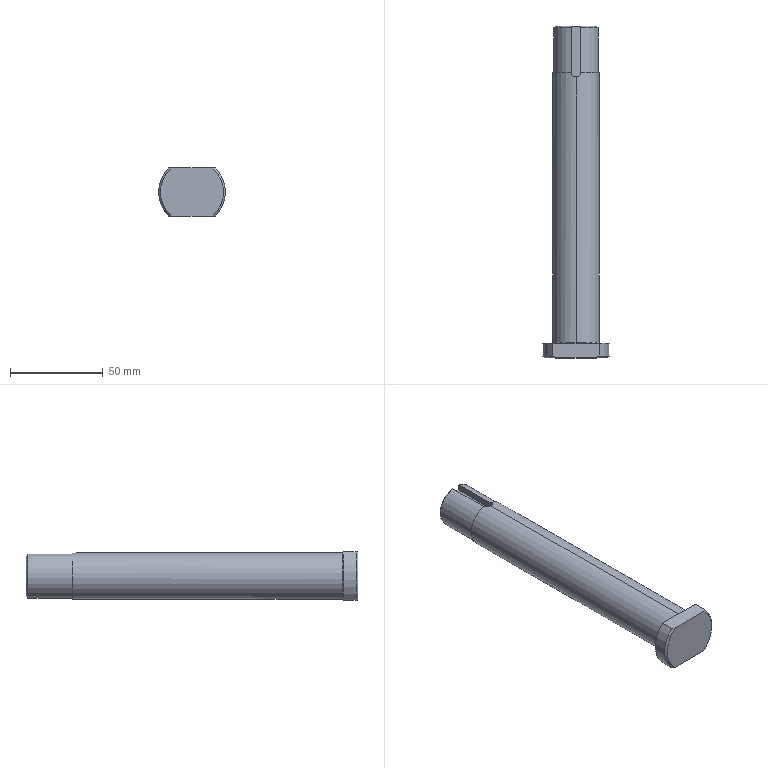Part | SolidWorks | features Chamfer 2, Fillet 2, ICE 2, Revolution 1 | 1 solid | 22 faces | box 36 x 179 x 26 mm | volume 89159 mm3 | plane 10 | cylinder 6 | cone 4 | torus 2 | commonest cylinder face diameters 25 x2 36 x2 5 x1 24 x1
STEP:
#1=CARTESIAN_POINT('',(0.,8.,13.));
#2=VERTEX_POINT('',#1);
#3=CARTESIAN_POINT('',(0.,8.,-13.));
#4=VERTEX_POINT('',#3);
#5=CARTESIAN_POINT('',(0.,8.,0.));
#6=DIRECTION('',(0.,-1.,0.));
#7=DIRECTION('',(0.,0.,-1.));
#8=AXIS2_PLACEMENT_3D('',#5,#6,#7);
#9=CIRCLE('',#8,13.);
#10=EDGE_CURVE('',#2,#4,#9,.T.);
#11=ORIENTED_EDGE('',*,*,#10,.F.);
#12=CARTESIAN_POINT('',(0.,8.5,12.5));
#13=VERTEX_POINT('',#12);
#14=CARTESIAN_POINT('',(0.,8.5,13.));
#15=DIRECTION('',(1.,0.,0.));
#16=DIRECTION('',(0.,0.,-1.));
#17=AXIS2_PLACEMENT_3D('',#14,#15,#16);
#18=CIRCLE('',#17,0.5);
#19=EDGE_CURVE('',#2,#13,#18,.T.);
#20=ORIENTED_EDGE('',*,*,#19,.T.);
#21=CARTESIAN_POINT('',(0.,8.5,-12.5));
#22=VERTEX_POINT('',#21);
#23=CARTESIAN_POINT('',(0.,8.5,0.));
#24=DIRECTION('',(0.,1.,0.));
#25=DIRECTION('',(0.,0.,-1.));
#26=AXIS2_PLACEMENT_3D('',#23,#24,#25);
#27=CIRCLE('',#26,12.5);
#28=EDGE_CURVE('',#22,#13,#27,.T.);
#29=ORIENTED_EDGE('',*,*,#28,.F.);
#30=CARTESIAN_POINT('',(0.,8.5,-13.));
#31=DIRECTION('',(-1.,0.,0.));
#32=DIRECTION('',(0.,0.,1.));
#33=AXIS2_PLACEMENT_3D('',#30,#31,#32);
#34=CIRCLE('',#33,0.5);
#35=EDGE_CURVE('',#4,#22,#34,.T.);
#36=ORIENTED_EDGE('',*,*,#35,.F.);
#37=EDGE_LOOP('',(#11,#20,#29,#36));
#38=FACE_OUTER_BOUND('',#37,.T.);
#39=CARTESIAN_POINT('',(0.,8.5,0.));
#40=DIRECTION('',(0.,-1.,0.));
#41=DIRECTION('',(0.,0.,-1.));
#42=AXIS2_PLACEMENT_3D('',#39,#40,#41);
#43=TOROIDAL_SURFACE('',#42,13.,0.5);
#44=ADVANCED_FACE('',(#38),#43,.F.);
#45=CARTESIAN_POINT('',(0.,179.,-11.));
#46=VERTEX_POINT('',#45);
#47=CARTESIAN_POINT('',(-2.5,179.,10.712));
#48=VERTEX_POINT('',#47);
#49=CARTESIAN_POINT('',(0.,179.,0.));
#50=DIRECTION('',(0.,1.,0.));
#51=DIRECTION('',(0.,0.,-1.));
#52=AXIS2_PLACEMENT_3D('',#49,#50,#51);
#53=CIRCLE('',#52,11.);
#54=EDGE_CURVE('',#46,#48,#53,.T.);
#55=ORIENTED_EDGE('',*,*,#54,.F.);
#56=CARTESIAN_POINT('',(0.,178.,-12.));
#57=VERTEX_POINT('',#56);
#58=CARTESIAN_POINT('',(0.,179.,-11.));
#59=DIRECTION('',(0.,-0.7071,-0.7071));
#60=VECTOR('',#59,1000.);
#61=LINE('',#58,#60);
#62=EDGE_CURVE('',#46,#57,#61,.T.);
#63=ORIENTED_EDGE('',*,*,#62,.T.);
#64=CARTESIAN_POINT('',(-2.5,178.,11.737));
#65=VERTEX_POINT('',#64);
#66=CARTESIAN_POINT('',(0.,178.,0.));
#67=DIRECTION('',(0.,-1.,0.));
#68=DIRECTION('',(0.,0.,-1.));
#69=AXIS2_PLACEMENT_3D('',#66,#67,#68);
#70=CIRCLE('',#69,12.);
#71=EDGE_CURVE('',#65,#57,#70,.T.);
#72=ORIENTED_EDGE('',*,*,#71,.F.);
#73=CARTESIAN_POINT('',(-2.5,179.,10.712));
#74=CARTESIAN_POINT('',(-2.5,178.667,11.054));
#75=CARTESIAN_POINT('',(-2.5,178.334,11.396));
#76=CARTESIAN_POINT('',(-2.5,178.,11.737));
#77=B_SPLINE_CURVE_WITH_KNOTS('',3,(#73,#74,#75,#76),.UNSPECIFIED.,.F.,.F.,(4,4),(0.,0.001432),.UNSPECIFIED.);
#78=EDGE_CURVE('',#48,#65,#77,.T.);
#79=ORIENTED_EDGE('',*,*,#78,.F.);
#80=EDGE_LOOP('',(#55,#63,#72,#79));
#81=FACE_OUTER_BOUND('',#80,.T.);
#82=CARTESIAN_POINT('',(0.,179.,0.));
#83=DIRECTION('',(0.,-1.,0.));
#84=DIRECTION('',(0.,0.,-1.));
#85=AXIS2_PLACEMENT_3D('',#82,#83,#84);
#86=CONICAL_SURFACE('',#85,11.,0.7854);
#87=ADVANCED_FACE('',(#81),#86,.T.);
#88=CARTESIAN_POINT('',(0.,8.5,0.));
#89=DIRECTION('',(0.,1.,0.));
#90=DIRECTION('',(0.,0.,-1.));
#91=AXIS2_PLACEMENT_3D('',#88,#89,#90);
#92=CIRCLE('',#91,12.5);
#93=EDGE_CURVE('',#13,#22,#92,.T.);
#94=ORIENTED_EDGE('',*,*,#93,.T.);
#95=CARTESIAN_POINT('',(0.,154.,-12.5));
#96=VERTEX_POINT('',#95);
#97=CARTESIAN_POINT('',(0.,0.,-12.5));
#98=DIRECTION('',(0.,1.,0.));
#99=VECTOR('',#98,1000.);
#100=LINE('',#97,#99);
#101=EDGE_CURVE('',#22,#96,#100,.T.);
#102=ORIENTED_EDGE('',*,*,#101,.T.);
#103=CARTESIAN_POINT('',(2.5,154.,12.247));
#104=VERTEX_POINT('',#103);
#105=CARTESIAN_POINT('',(0.,154.,0.));
#106=DIRECTION('',(0.,1.,0.));
#107=DIRECTION('',(0.,0.,1.));
#108=AXIS2_PLACEMENT_3D('',#105,#106,#107);
#109=CIRCLE('',#108,12.5);
#110=EDGE_CURVE('',#104,#96,#109,.T.);
#111=ORIENTED_EDGE('',*,*,#110,.F.);
#112=CARTESIAN_POINT('',(0.,151.5,12.5));
#113=VERTEX_POINT('',#112);
#114=CARTESIAN_POINT('',(2.5,154.,12.247));
#115=CARTESIAN_POINT('',(2.5,153.834,12.247));
#116=CARTESIAN_POINT('',(2.484,153.672,12.251));
#117=CARTESIAN_POINT('',(2.42,153.351,12.264));
#118=CARTESIAN_POINT('',(2.372,153.192,12.273));
#119=CARTESIAN_POINT('',(2.246,152.89,12.297));
#120=CARTESIAN_POINT('',(2.169,152.746,12.311));
#121=CARTESIAN_POINT('',(1.987,152.475,12.341));
#122=CARTESIAN_POINT('',(1.882,152.346,12.358));
#123=CARTESIAN_POINT('',(1.537,152.002,12.407));
#124=CARTESIAN_POINT('',(1.258,151.815,12.44));
#125=CARTESIAN_POINT('',(0.8073,151.628,12.475));
#126=CARTESIAN_POINT('',(0.6491,151.58,12.484));
#127=CARTESIAN_POINT('',(0.3261,151.516,12.497));
#128=CARTESIAN_POINT('',(0.1636,151.5,12.5));
#129=CARTESIAN_POINT('',(0.,151.5,12.5));
#130=B_SPLINE_CURVE_WITH_KNOTS('',3,(#114,#115,#116,#117,#118,#119,#120,#121,#122,#123,#124,#125,#126,#127,#128,#129),.UNSPECIFIED.,.F.,.F.,(4,2,2,2,2,2,2,4),(0.,0.0004899,0.0009797,0.00147,0.001959,0.002939,0.003429,0.003919),.UNSPECIFIED.);
#131=EDGE_CURVE('',#104,#113,#130,.T.);
#132=ORIENTED_EDGE('',*,*,#131,.T.);
#133=CARTESIAN_POINT('',(0.,0.,12.5));
#134=DIRECTION('',(0.,1.,0.));
#135=VECTOR('',#134,1000.);
#136=LINE('',#133,#135);
#137=EDGE_CURVE('',#13,#113,#136,.T.);
#138=ORIENTED_EDGE('',*,*,#137,.F.);
#139=EDGE_LOOP('',(#94,#102,#111,#132,#138));
#140=FACE_OUTER_BOUND('',#139,.T.);
#141=CARTESIAN_POINT('',(0.,0.,0.));
#142=DIRECTION('',(0.,1.,0.));
#143=DIRECTION('',(0.,0.,1.));
#144=AXIS2_PLACEMENT_3D('',#141,#142,#143);
#145=CYLINDRICAL_SURFACE('',#144,12.5);
#146=ADVANCED_FACE('',(#140),#145,.T.);
#147=CARTESIAN_POINT('',(-12.45,8.,13.));
#148=VERTEX_POINT('',#147);
#149=CARTESIAN_POINT('',(18.,8.,13.));
#150=DIRECTION('',(1.,0.,0.));
#151=VECTOR('',#150,1000.);
#152=LINE('',#149,#151);
#153=EDGE_CURVE('',#148,#2,#152,.T.);
#154=ORIENTED_EDGE('',*,*,#153,.T.);
#155=ORIENTED_EDGE('',*,*,#10,.T.);
#156=CARTESIAN_POINT('',(-12.45,8.,-13.));
#157=VERTEX_POINT('',#156);
#158=CARTESIAN_POINT('',(18.,8.,-13.));
#159=DIRECTION('',(-1.,0.,0.));
#160=VECTOR('',#159,1000.);
#161=LINE('',#158,#160);
#162=EDGE_CURVE('',#4,#157,#161,.T.);
#163=ORIENTED_EDGE('',*,*,#162,.T.);
#164=CARTESIAN_POINT('',(0.,8.,0.));
#165=DIRECTION('',(0.,1.,0.));
#166=DIRECTION('',(0.,0.,1.));
#167=AXIS2_PLACEMENT_3D('',#164,#165,#166);
#168=CIRCLE('',#167,18.);
#169=EDGE_CURVE('',#157,#148,#168,.T.);
#170=ORIENTED_EDGE('',*,*,#169,.T.);
#171=EDGE_LOOP('',(#154,#155,#163,#170));
#172=FACE_OUTER_BOUND('',#171,.T.);
#173=CARTESIAN_POINT('',(18.,8.,0.));
#174=DIRECTION('',(0.,-1.,0.));
#175=DIRECTION('',(0.,0.,-1.));
#176=AXIS2_PLACEMENT_3D('',#173,#174,#175);
#177=PLANE('',#176);
#178=ADVANCED_FACE('',(#172),#177,.F.);
#179=ORIENTED_EDGE('',*,*,#101,.F.);
#180=ORIENTED_EDGE('',*,*,#28,.T.);
#181=ORIENTED_EDGE('',*,*,#137,.T.);
#182=CARTESIAN_POINT('',(-2.5,154.,12.247));
#183=VERTEX_POINT('',#182);
#184=CARTESIAN_POINT('',(0.,151.5,12.5));
#185=CARTESIAN_POINT('',(-0.1634,151.5,12.5));
#186=CARTESIAN_POINT('',(-0.3294,151.516,12.497));
#187=CARTESIAN_POINT('',(-0.6501,151.58,12.484));
#188=CARTESIAN_POINT('',(-0.806,151.628,12.475));
#189=CARTESIAN_POINT('',(-1.109,151.753,12.452));
#190=CARTESIAN_POINT('',(-1.255,151.832,12.438));
#191=CARTESIAN_POINT('',(-1.525,152.012,12.407));
#192=CARTESIAN_POINT('',(-1.651,152.116,12.391));
#193=CARTESIAN_POINT('',(-1.884,152.348,12.358));
#194=CARTESIAN_POINT('',(-1.987,152.474,12.341));
#195=CARTESIAN_POINT('',(-2.168,152.744,12.311));
#196=CARTESIAN_POINT('',(-2.246,152.89,12.297));
#197=CARTESIAN_POINT('',(-2.371,153.192,12.273));
#198=CARTESIAN_POINT('',(-2.419,153.348,12.264));
#199=CARTESIAN_POINT('',(-2.483,153.669,12.251));
#200=CARTESIAN_POINT('',(-2.5,153.834,12.247));
#201=CARTESIAN_POINT('',(-2.5,154.,12.247));
#202=B_SPLINE_CURVE_WITH_KNOTS('',3,(#184,#185,#186,#187,#188,#189,#190,#191,#192,#193,#194,#195,#196,#197,#198,#199,#200,#201),.UNSPECIFIED.,.F.,.F.,(4,2,2,2,2,2,2,2,4),(0.003919,0.004408,0.004898,0.005387,0.005876,0.006366,0.006855,0.007344,0.007834),.UNSPECIFIED.);
#203=EDGE_CURVE('',#113,#183,#202,.T.);
#204=ORIENTED_EDGE('',*,*,#203,.T.);
#205=CARTESIAN_POINT('',(0.,154.,0.));
#206=DIRECTION('',(0.,1.,0.));
#207=DIRECTION('',(0.,0.,1.));
#208=AXIS2_PLACEMENT_3D('',#205,#206,#207);
#209=CIRCLE('',#208,12.5);
#210=EDGE_CURVE('',#96,#183,#209,.T.);
#211=ORIENTED_EDGE('',*,*,#210,.F.);
#212=EDGE_LOOP('',(#179,#180,#181,#204,#211));
#213=FACE_OUTER_BOUND('',#212,.T.);
#214=CARTESIAN_POINT('',(0.,0.,0.));
#215=DIRECTION('',(0.,1.,0.));
#216=DIRECTION('',(0.,0.,1.));
#217=AXIS2_PLACEMENT_3D('',#214,#215,#216);
#218=CYLINDRICAL_SURFACE('',#217,12.5);
#219=ADVANCED_FACE('',(#213),#218,.T.);
#220=CARTESIAN_POINT('',(-2.5,154.,11.737));
#221=VERTEX_POINT('',#220);
#222=CARTESIAN_POINT('',(-2.5,154.,13.001));
#223=DIRECTION('',(0.,0.,-1.));
#224=VECTOR('',#223,1000.);
#225=LINE('',#222,#224);
#226=EDGE_CURVE('',#183,#221,#225,.T.);
#227=ORIENTED_EDGE('',*,*,#226,.T.);
#228=CARTESIAN_POINT('',(2.5,154.,11.737));
#229=VERTEX_POINT('',#228);
#230=CARTESIAN_POINT('',(0.,154.,0.));
#231=DIRECTION('',(0.,1.,0.));
#232=DIRECTION('',(0.,0.,1.));
#233=AXIS2_PLACEMENT_3D('',#230,#231,#232);
#234=CIRCLE('',#233,12.);
#235=EDGE_CURVE('',#229,#221,#234,.T.);
#236=ORIENTED_EDGE('',*,*,#235,.F.);
#237=CARTESIAN_POINT('',(2.5,154.,13.001));
#238=DIRECTION('',(0.,0.,-1.));
#239=VECTOR('',#238,1000.);
#240=LINE('',#237,#239);
#241=EDGE_CURVE('',#104,#229,#240,.T.);
#242=ORIENTED_EDGE('',*,*,#241,.F.);
#243=ORIENTED_EDGE('',*,*,#110,.T.);
#244=ORIENTED_EDGE('',*,*,#210,.T.);
#245=EDGE_LOOP('',(#227,#236,#242,#243,#244));
#246=FACE_OUTER_BOUND('',#245,.T.);
#247=CARTESIAN_POINT('',(12.5,154.,0.));
#248=DIRECTION('',(0.,-1.,0.));
#249=DIRECTION('',(0.,0.,-1.));
#250=AXIS2_PLACEMENT_3D('',#247,#248,#249);
#251=PLANE('',#250);
#252=ADVANCED_FACE('',(#246),#251,.F.);
#253=CARTESIAN_POINT('',(-2.5,0.,11.737));
#254=DIRECTION('',(0.,1.,0.));
#255=VECTOR('',#254,1000.);
#256=LINE('',#253,#255);
#257=EDGE_CURVE('',#221,#65,#256,.T.);
#258=ORIENTED_EDGE('',*,*,#257,.T.);
#259=ORIENTED_EDGE('',*,*,#71,.T.);
#260=CARTESIAN_POINT('',(2.5,178.,11.737));
#261=VERTEX_POINT('',#260);
#262=CARTESIAN_POINT('',(0.,178.,0.));
#263=DIRECTION('',(0.,-1.,0.));
#264=DIRECTION('',(0.,0.,-1.));
#265=AXIS2_PLACEMENT_3D('',#262,#263,#264);
#266=CIRCLE('',#265,12.);
#267=EDGE_CURVE('',#57,#261,#266,.T.);
#268=ORIENTED_EDGE('',*,*,#267,.T.);
#269=CARTESIAN_POINT('',(2.5,0.,11.737));
#270=DIRECTION('',(0.,-1.,0.));
#271=VECTOR('',#270,1000.);
#272=LINE('',#269,#271);
#273=EDGE_CURVE('',#261,#229,#272,.T.);
#274=ORIENTED_EDGE('',*,*,#273,.T.);
#275=ORIENTED_EDGE('',*,*,#235,.T.);
#276=EDGE_LOOP('',(#258,#259,#268,#274,#275));
#277=FACE_OUTER_BOUND('',#276,.T.);
#278=CARTESIAN_POINT('',(0.,0.,0.));
#279=DIRECTION('',(0.,1.,0.));
#280=DIRECTION('',(0.,0.,1.));
#281=AXIS2_PLACEMENT_3D('',#278,#279,#280);
#282=CYLINDRICAL_SURFACE('',#281,12.);
#283=ADVANCED_FACE('',(#277),#282,.T.);
#284=CARTESIAN_POINT('',(2.5,179.,8.));
#285=VERTEX_POINT('',#284);
#286=CARTESIAN_POINT('',(2.5,179.,10.712));
#287=VERTEX_POINT('',#286);
#288=CARTESIAN_POINT('',(2.5,179.,13.001));
#289=DIRECTION('',(0.,0.,1.));
#290=VECTOR('',#289,1000.);
#291=LINE('',#288,#290);
#292=EDGE_CURVE('',#285,#287,#291,.T.);
#293=ORIENTED_EDGE('',*,*,#292,.T.);
#294=CARTESIAN_POINT('',(0.,179.,0.));
#295=DIRECTION('',(0.,1.,0.));
#296=DIRECTION('',(0.,0.,-1.));
#297=AXIS2_PLACEMENT_3D('',#294,#295,#296);
#298=CIRCLE('',#297,11.);
#299=EDGE_CURVE('',#287,#46,#298,.T.);
#300=ORIENTED_EDGE('',*,*,#299,.T.);
#301=ORIENTED_EDGE('',*,*,#54,.T.);
#302=CARTESIAN_POINT('',(-2.5,179.,8.));
#303=VERTEX_POINT('',#302);
#304=CARTESIAN_POINT('',(-2.5,179.,13.001));
#305=DIRECTION('',(0.,0.,-1.));
#306=VECTOR('',#305,1000.);
#307=LINE('',#304,#306);
#308=EDGE_CURVE('',#48,#303,#307,.T.);
#309=ORIENTED_EDGE('',*,*,#308,.T.);
#310=CARTESIAN_POINT('',(0.,179.,8.));
#311=DIRECTION('',(1.,0.,0.));
#312=VECTOR('',#311,1000.);
#313=LINE('',#310,#312);
#314=EDGE_CURVE('',#303,#285,#313,.T.);
#315=ORIENTED_EDGE('',*,*,#314,.T.);
#316=EDGE_LOOP('',(#293,#300,#301,#309,#315));
#317=FACE_OUTER_BOUND('',#316,.T.);
#318=CARTESIAN_POINT('',(12.,179.,0.));
#319=DIRECTION('',(0.,-1.,0.));
#320=DIRECTION('',(0.,0.,-1.));
#321=AXIS2_PLACEMENT_3D('',#318,#319,#320);
#322=PLANE('',#321);
#323=ADVANCED_FACE('',(#317),#322,.F.);
#324=CARTESIAN_POINT('',(-12.45,1.,-13.));
#325=VERTEX_POINT('',#324);
#326=CARTESIAN_POINT('',(-12.45,0.,-13.));
#327=DIRECTION('',(0.,-1.,0.));
#328=VECTOR('',#327,1000.);
#329=LINE('',#326,#328);
#330=EDGE_CURVE('',#157,#325,#329,.T.);
#331=ORIENTED_EDGE('',*,*,#330,.T.);
#332=CARTESIAN_POINT('',(-12.45,1.,13.));
#333=VERTEX_POINT('',#332);
#334=CARTESIAN_POINT('',(0.,1.,0.));
#335=DIRECTION('',(0.,1.,0.));
#336=DIRECTION('',(0.,0.,1.));
#337=AXIS2_PLACEMENT_3D('',#334,#335,#336);
#338=CIRCLE('',#337,18.);
#339=EDGE_CURVE('',#325,#333,#338,.T.);
#340=ORIENTED_EDGE('',*,*,#339,.T.);
#341=CARTESIAN_POINT('',(-12.45,0.,13.));
#342=DIRECTION('',(0.,1.,0.));
#343=VECTOR('',#342,1000.);
#344=LINE('',#341,#343);
#345=EDGE_CURVE('',#333,#148,#344,.T.);
#346=ORIENTED_EDGE('',*,*,#345,.T.);
#347=ORIENTED_EDGE('',*,*,#169,.F.);
#348=EDGE_LOOP('',(#331,#340,#346,#347));
#349=FACE_OUTER_BOUND('',#348,.T.);
#350=CARTESIAN_POINT('',(0.,0.,0.));
#351=DIRECTION('',(0.,1.,0.));
#352=DIRECTION('',(0.,0.,1.));
#353=AXIS2_PLACEMENT_3D('',#350,#351,#352);
#354=CYLINDRICAL_SURFACE('',#353,18.);
#355=ADVANCED_FACE('',(#349),#354,.T.);
#356=CARTESIAN_POINT('',(-10.954,0.,13.));
#357=VERTEX_POINT('',#356);
#358=CARTESIAN_POINT('',(10.954,0.,13.));
#359=VERTEX_POINT('',#358);
#360=CARTESIAN_POINT('',(65.,0.,13.));
#361=DIRECTION('',(1.,0.,0.));
#362=VECTOR('',#361,1000.);
#363=LINE('',#360,#362);
#364=EDGE_CURVE('',#357,#359,#363,.T.);
#365=ORIENTED_EDGE('',*,*,#364,.F.);
#366=CARTESIAN_POINT('',(-10.954,0.,-13.));
#367=VERTEX_POINT('',#366);
#368=CARTESIAN_POINT('',(0.,0.,0.));
#369=DIRECTION('',(0.,-1.,0.));
#370=DIRECTION('',(0.,0.,1.));
#371=AXIS2_PLACEMENT_3D('',#368,#369,#370);
#372=CIRCLE('',#371,17.);
#373=EDGE_CURVE('',#357,#367,#372,.T.);
#374=ORIENTED_EDGE('',*,*,#373,.T.);
#375=CARTESIAN_POINT('',(10.954,0.,-13.));
#376=VERTEX_POINT('',#375);
#377=CARTESIAN_POINT('',(65.,0.,-13.));
#378=DIRECTION('',(-1.,0.,0.));
#379=VECTOR('',#378,1000.);
#380=LINE('',#377,#379);
#381=EDGE_CURVE('',#376,#367,#380,.T.);
#382=ORIENTED_EDGE('',*,*,#381,.F.);
#383=CARTESIAN_POINT('',(0.,0.,0.));
#384=DIRECTION('',(0.,-1.,0.));
#385=DIRECTION('',(0.,0.,1.));
#386=AXIS2_PLACEMENT_3D('',#383,#384,#385);
#387=CIRCLE('',#386,17.);
#388=EDGE_CURVE('',#376,#359,#387,.T.);
#389=ORIENTED_EDGE('',*,*,#388,.T.);
#390=EDGE_LOOP('',(#365,#374,#382,#389));
#391=FACE_OUTER_BOUND('',#390,.T.);
#392=CARTESIAN_POINT('',(0.,0.,0.));
#393=DIRECTION('',(0.,1.,0.));
#394=DIRECTION('',(0.,0.,1.));
#395=AXIS2_PLACEMENT_3D('',#392,#393,#394);
#396=PLANE('',#395);
#397=ADVANCED_FACE('',(#391),#396,.F.);
#398=CARTESIAN_POINT('',(12.45,8.,13.));
#399=VERTEX_POINT('',#398);
#400=CARTESIAN_POINT('',(12.45,1.,13.));
#401=VERTEX_POINT('',#400);
#402=CARTESIAN_POINT('',(12.45,0.,13.));
#403=DIRECTION('',(0.,-1.,0.));
#404=VECTOR('',#403,1000.);
#405=LINE('',#402,#404);
#406=EDGE_CURVE('',#399,#401,#405,.T.);
#407=ORIENTED_EDGE('',*,*,#406,.T.);
#408=CARTESIAN_POINT('',(12.45,1.,-13.));
#409=VERTEX_POINT('',#408);
#410=CARTESIAN_POINT('',(0.,1.,0.));
#411=DIRECTION('',(0.,1.,0.));
#412=DIRECTION('',(0.,0.,1.));
#413=AXIS2_PLACEMENT_3D('',#410,#411,#412);
#414=CIRCLE('',#413,18.);
#415=EDGE_CURVE('',#401,#409,#414,.T.);
#416=ORIENTED_EDGE('',*,*,#415,.T.);
#417=CARTESIAN_POINT('',(12.45,8.,-13.));
#418=VERTEX_POINT('',#417);
#419=CARTESIAN_POINT('',(12.45,0.,-13.));
#420=DIRECTION('',(0.,1.,0.));
#421=VECTOR('',#420,1000.);
#422=LINE('',#419,#421);
#423=EDGE_CURVE('',#409,#418,#422,.T.);
#424=ORIENTED_EDGE('',*,*,#423,.T.);
#425=CARTESIAN_POINT('',(0.,8.,0.));
#426=DIRECTION('',(0.,1.,0.));
#427=DIRECTION('',(0.,0.,1.));
#428=AXIS2_PLACEMENT_3D('',#425,#426,#427);
#429=CIRCLE('',#428,18.);
#430=EDGE_CURVE('',#399,#418,#429,.T.);
#431=ORIENTED_EDGE('',*,*,#430,.F.);
#432=EDGE_LOOP('',(#407,#416,#424,#431));
#433=FACE_OUTER_BOUND('',#432,.T.);
#434=CARTESIAN_POINT('',(0.,0.,0.));
#435=DIRECTION('',(0.,1.,0.));
#436=DIRECTION('',(0.,0.,1.));
#437=AXIS2_PLACEMENT_3D('',#434,#435,#436);
#438=CYLINDRICAL_SURFACE('',#437,18.);
#439=ADVANCED_FACE('',(#433),#438,.T.);
#440=CARTESIAN_POINT('',(18.,8.,-13.));
#441=DIRECTION('',(-1.,0.,0.));
#442=VECTOR('',#441,1000.);
#443=LINE('',#440,#442);
#444=EDGE_CURVE('',#418,#4,#443,.T.);
#445=ORIENTED_EDGE('',*,*,#444,.T.);
#446=CARTESIAN_POINT('',(0.,8.,0.));
#447=DIRECTION('',(0.,-1.,0.));
#448=DIRECTION('',(0.,0.,-1.));
#449=AXIS2_PLACEMENT_3D('',#446,#447,#448);
#450=CIRCLE('',#449,13.);
#451=EDGE_CURVE('',#4,#2,#450,.T.);
#452=ORIENTED_EDGE('',*,*,#451,.T.);
#453=CARTESIAN_POINT('',(18.,8.,13.));
#454=DIRECTION('',(1.,0.,0.));
#455=VECTOR('',#454,1000.);
#456=LINE('',#453,#455);
#457=EDGE_CURVE('',#2,#399,#456,.T.);
#458=ORIENTED_EDGE('',*,*,#457,.T.);
#459=ORIENTED_EDGE('',*,*,#430,.T.);
#460=EDGE_LOOP('',(#445,#452,#458,#459));
#461=FACE_OUTER_BOUND('',#460,.T.);
#462=CARTESIAN_POINT('',(18.,8.,0.));
#463=DIRECTION('',(0.,-1.,0.));
#464=DIRECTION('',(0.,0.,-1.));
#465=AXIS2_PLACEMENT_3D('',#462,#463,#464);
#466=PLANE('',#465);
#467=ADVANCED_FACE('',(#461),#466,.F.);
#468=ORIENTED_EDGE('',*,*,#381,.T.);
#469=CARTESIAN_POINT('',(-10.954,0.,-13.));
#470=CARTESIAN_POINT('',(-11.459,0.3249,-13.));
#471=CARTESIAN_POINT('',(-11.957,0.6588,-13.));
#472=CARTESIAN_POINT('',(-12.45,1.,-13.));
#473=B_SPLINE_CURVE_WITH_KNOTS('',3,(#469,#470,#471,#472),.UNSPECIFIED.,.F.,.F.,(4,4),(0.,0.001799),.UNSPECIFIED.);
#474=EDGE_CURVE('',#367,#325,#473,.T.);
#475=ORIENTED_EDGE('',*,*,#474,.T.);
#476=ORIENTED_EDGE('',*,*,#330,.F.);
#477=ORIENTED_EDGE('',*,*,#162,.F.);
#478=ORIENTED_EDGE('',*,*,#444,.F.);
#479=ORIENTED_EDGE('',*,*,#423,.F.);
#480=CARTESIAN_POINT('',(12.45,1.,-13.));
#481=CARTESIAN_POINT('',(11.957,0.6588,-13.));
#482=CARTESIAN_POINT('',(11.459,0.3249,-13.));
#483=CARTESIAN_POINT('',(10.954,0.,-13.));
#484=B_SPLINE_CURVE_WITH_KNOTS('',3,(#480,#481,#482,#483),.UNSPECIFIED.,.F.,.F.,(4,4),(0.,0.001799),.UNSPECIFIED.);
#485=EDGE_CURVE('',#409,#376,#484,.T.);
#486=ORIENTED_EDGE('',*,*,#485,.T.);
#487=EDGE_LOOP('',(#468,#475,#476,#477,#478,#479,#486));
#488=FACE_OUTER_BOUND('',#487,.T.);
#489=CARTESIAN_POINT('',(65.,10.,-13.));
#490=DIRECTION('',(0.,0.,1.));
#491=DIRECTION('',(1.,0.,0.));
#492=AXIS2_PLACEMENT_3D('',#489,#490,#491);
#493=PLANE('',#492);
#494=ADVANCED_FACE('',(#488),#493,.F.);
#495=ORIENTED_EDGE('',*,*,#345,.F.);
#496=CARTESIAN_POINT('',(-12.45,1.,13.));
#497=CARTESIAN_POINT('',(-11.957,0.6588,13.));
#498=CARTESIAN_POINT('',(-11.459,0.3249,13.));
#499=CARTESIAN_POINT('',(-10.954,0.,13.));
#500=B_SPLINE_CURVE_WITH_KNOTS('',3,(#496,#497,#498,#499),.UNSPECIFIED.,.F.,.F.,(4,4),(0.,0.001799),.UNSPECIFIED.);
#501=EDGE_CURVE('',#333,#357,#500,.T.);
#502=ORIENTED_EDGE('',*,*,#501,.T.);
#503=ORIENTED_EDGE('',*,*,#364,.T.);
#504=CARTESIAN_POINT('',(10.954,0.,13.));
#505=CARTESIAN_POINT('',(11.459,0.3249,13.));
#506=CARTESIAN_POINT('',(11.957,0.6588,13.));
#507=CARTESIAN_POINT('',(12.45,1.,13.));
#508=B_SPLINE_CURVE_WITH_KNOTS('',3,(#504,#505,#506,#507),.UNSPECIFIED.,.F.,.F.,(4,4),(0.,0.001799),.UNSPECIFIED.);
#509=EDGE_CURVE('',#359,#401,#508,.T.);
#510=ORIENTED_EDGE('',*,*,#509,.T.);
#511=ORIENTED_EDGE('',*,*,#406,.F.);
#512=ORIENTED_EDGE('',*,*,#457,.F.);
#513=ORIENTED_EDGE('',*,*,#153,.F.);
#514=EDGE_LOOP('',(#495,#502,#503,#510,#511,#512,#513));
#515=FACE_OUTER_BOUND('',#514,.T.);
#516=CARTESIAN_POINT('',(65.,10.,13.));
#517=DIRECTION('',(0.,0.,-1.));
#518=DIRECTION('',(-1.,0.,0.));
#519=AXIS2_PLACEMENT_3D('',#516,#517,#518);
#520=PLANE('',#519);
#521=ADVANCED_FACE('',(#515),#520,.F.);
#522=ORIENTED_EDGE('',*,*,#308,.F.);
#523=ORIENTED_EDGE('',*,*,#78,.T.);
#524=ORIENTED_EDGE('',*,*,#257,.F.);
#525=CARTESIAN_POINT('',(-2.5,154.,8.));
#526=VERTEX_POINT('',#525);
#527=CARTESIAN_POINT('',(-2.5,154.,13.001));
#528=DIRECTION('',(0.,0.,-1.));
#529=VECTOR('',#528,1000.);
#530=LINE('',#527,#529);
#531=EDGE_CURVE('',#221,#526,#530,.T.);
#532=ORIENTED_EDGE('',*,*,#531,.T.);
#533=CARTESIAN_POINT('',(-2.5,179.,8.));
#534=DIRECTION('',(0.,-1.,0.));
#535=VECTOR('',#534,1000.);
#536=LINE('',#533,#535);
#537=EDGE_CURVE('',#303,#526,#536,.T.);
#538=ORIENTED_EDGE('',*,*,#537,.F.);
#539=EDGE_LOOP('',(#522,#523,#524,#532,#538));
#540=FACE_OUTER_BOUND('',#539,.T.);
#541=CARTESIAN_POINT('',(-2.5,179.,13.001));
#542=DIRECTION('',(1.,0.,0.));
#543=DIRECTION('',(0.,1.,0.));
#544=AXIS2_PLACEMENT_3D('',#541,#542,#543);
#545=PLANE('',#544);
#546=ADVANCED_FACE('',(#540),#545,.T.);
#547=ORIENTED_EDGE('',*,*,#241,.T.);
#548=CARTESIAN_POINT('',(2.5,154.,8.));
#549=VERTEX_POINT('',#548);
#550=CARTESIAN_POINT('',(2.5,154.,13.001));
#551=DIRECTION('',(0.,0.,-1.));
#552=VECTOR('',#551,1000.);
#553=LINE('',#550,#552);
#554=EDGE_CURVE('',#229,#549,#553,.T.);
#555=ORIENTED_EDGE('',*,*,#554,.T.);
#556=CARTESIAN_POINT('',(0.,154.,8.));
#557=DIRECTION('',(0.,0.,1.));
#558=DIRECTION('',(1.,0.,0.));
#559=AXIS2_PLACEMENT_3D('',#556,#557,#558);
#560=CIRCLE('',#559,2.5);
#561=EDGE_CURVE('',#526,#549,#560,.T.);
#562=ORIENTED_EDGE('',*,*,#561,.F.);
#563=ORIENTED_EDGE('',*,*,#531,.F.);
#564=ORIENTED_EDGE('',*,*,#226,.F.);
#565=ORIENTED_EDGE('',*,*,#203,.F.);
#566=ORIENTED_EDGE('',*,*,#131,.F.);
#567=EDGE_LOOP('',(#547,#555,#562,#563,#564,#565,#566));
#568=FACE_OUTER_BOUND('',#567,.T.);
#569=CARTESIAN_POINT('',(0.,154.,13.001));
#570=DIRECTION('',(0.,0.,-1.));
#571=DIRECTION('',(-1.,0.,0.));
#572=AXIS2_PLACEMENT_3D('',#569,#570,#571);
#573=CYLINDRICAL_SURFACE('',#572,2.5);
#574=ADVANCED_FACE('',(#568),#573,.F.);
#575=ORIENTED_EDGE('',*,*,#273,.F.);
#576=CARTESIAN_POINT('',(2.5,178.,11.737));
#577=CARTESIAN_POINT('',(2.5,178.334,11.396));
#578=CARTESIAN_POINT('',(2.5,178.667,11.054));
#579=CARTESIAN_POINT('',(2.5,179.,10.712));
#580=B_SPLINE_CURVE_WITH_KNOTS('',3,(#576,#577,#578,#579),.UNSPECIFIED.,.F.,.F.,(4,4),(0.,0.001432),.UNSPECIFIED.);
#581=EDGE_CURVE('',#261,#287,#580,.T.);
#582=ORIENTED_EDGE('',*,*,#581,.T.);
#583=ORIENTED_EDGE('',*,*,#292,.F.);
#584=CARTESIAN_POINT('',(2.5,179.,8.));
#585=DIRECTION('',(0.,1.,0.));
#586=VECTOR('',#585,1000.);
#587=LINE('',#584,#586);
#588=EDGE_CURVE('',#549,#285,#587,.T.);
#589=ORIENTED_EDGE('',*,*,#588,.F.);
#590=ORIENTED_EDGE('',*,*,#554,.F.);
#591=EDGE_LOOP('',(#575,#582,#583,#589,#590));
#592=FACE_OUTER_BOUND('',#591,.T.);
#593=CARTESIAN_POINT('',(2.5,179.,13.001));
#594=DIRECTION('',(-1.,0.,0.));
#595=DIRECTION('',(0.,-1.,0.));
#596=AXIS2_PLACEMENT_3D('',#593,#594,#595);
#597=PLANE('',#596);
#598=ADVANCED_FACE('',(#592),#597,.T.);
#599=ORIENTED_EDGE('',*,*,#537,.T.);
#600=ORIENTED_EDGE('',*,*,#561,.T.);
#601=ORIENTED_EDGE('',*,*,#588,.T.);
#602=ORIENTED_EDGE('',*,*,#314,.F.);
#603=EDGE_LOOP('',(#599,#600,#601,#602));
#604=FACE_OUTER_BOUND('',#603,.T.);
#605=CARTESIAN_POINT('',(0.,179.,8.));
#606=DIRECTION('',(0.,0.,1.));
#607=DIRECTION('',(1.,0.,0.));
#608=AXIS2_PLACEMENT_3D('',#605,#606,#607);
#609=PLANE('',#608);
#610=ADVANCED_FACE('',(#604),#609,.T.);
#611=ORIENTED_EDGE('',*,*,#62,.F.);
#612=ORIENTED_EDGE('',*,*,#299,.F.);
#613=ORIENTED_EDGE('',*,*,#581,.F.);
#614=ORIENTED_EDGE('',*,*,#267,.F.);
#615=EDGE_LOOP('',(#611,#612,#613,#614));
#616=FACE_OUTER_BOUND('',#615,.T.);
#617=CARTESIAN_POINT('',(0.,179.,0.));
#618=DIRECTION('',(0.,-1.,0.));
#619=DIRECTION('',(0.,0.,-1.));
#620=AXIS2_PLACEMENT_3D('',#617,#618,#619);
#621=CONICAL_SURFACE('',#620,11.,0.7854);
#622=ADVANCED_FACE('',(#616),#621,.T.);
#623=ORIENTED_EDGE('',*,*,#19,.F.);
#624=ORIENTED_EDGE('',*,*,#451,.F.);
#625=ORIENTED_EDGE('',*,*,#35,.T.);
#626=ORIENTED_EDGE('',*,*,#93,.F.);
#627=EDGE_LOOP('',(#623,#624,#625,#626));
#628=FACE_OUTER_BOUND('',#627,.T.);
#629=CARTESIAN_POINT('',(0.,8.5,0.));
#630=DIRECTION('',(0.,-1.,0.));
#631=DIRECTION('',(0.,0.,-1.));
#632=AXIS2_PLACEMENT_3D('',#629,#630,#631);
#633=TOROIDAL_SURFACE('',#632,13.,0.5);
#634=ADVANCED_FACE('',(#628),#633,.F.);
#635=ORIENTED_EDGE('',*,*,#474,.F.);
#636=ORIENTED_EDGE('',*,*,#373,.F.);
#637=ORIENTED_EDGE('',*,*,#501,.F.);
#638=ORIENTED_EDGE('',*,*,#339,.F.);
#639=EDGE_LOOP('',(#635,#636,#637,#638));
#640=FACE_OUTER_BOUND('',#639,.T.);
#641=CARTESIAN_POINT('',(0.,1.,0.));
#642=DIRECTION('',(0.,1.,0.));
#643=DIRECTION('',(0.,0.,1.));
#644=AXIS2_PLACEMENT_3D('',#641,#642,#643);
#645=CONICAL_SURFACE('',#644,18.,0.7854);
#646=ADVANCED_FACE('',(#640),#645,.T.);
#647=ORIENTED_EDGE('',*,*,#509,.F.);
#648=ORIENTED_EDGE('',*,*,#388,.F.);
#649=ORIENTED_EDGE('',*,*,#485,.F.);
#650=ORIENTED_EDGE('',*,*,#415,.F.);
#651=EDGE_LOOP('',(#647,#648,#649,#650));
#652=FACE_OUTER_BOUND('',#651,.T.);
#653=CARTESIAN_POINT('',(0.,1.,0.));
#654=DIRECTION('',(0.,1.,0.));
#655=DIRECTION('',(0.,0.,1.));
#656=AXIS2_PLACEMENT_3D('',#653,#654,#655);
#657=CONICAL_SURFACE('',#656,18.,0.7854);
#658=ADVANCED_FACE('',(#652),#657,.T.);
#659=CLOSED_SHELL('',(#44,#87,#146,#178,#219,#252,#283,#323,#355,#397,#439,#467,#494,#521,#546,#574,#598,#610,#622,#634,#646,#658));
#660=MANIFOLD_SOLID_BREP('',#659);
#661=CARTESIAN_POINT('',(0.,0.,0.));
#662=DIRECTION('',(0.,0.,1.));
#663=DIRECTION('',(1.,0.,0.));
#664=AXIS2_PLACEMENT_3D('',#661,#662,#663);
#665=(LENGTH_UNIT()NAMED_UNIT(*)SI_UNIT(.MILLI.,.METRE.));
#666=UNCERTAINTY_MEASURE_WITH_UNIT(LENGTH_MEASURE(0.00001),#665,'','');
#667=(NAMED_UNIT(*)PLANE_ANGLE_UNIT()SI_UNIT($,.RADIAN.));
#668=(NAMED_UNIT(*)SI_UNIT($,.STERADIAN.)SOLID_ANGLE_UNIT());
#669=(GEOMETRIC_REPRESENTATION_CONTEXT(3)GLOBAL_UNCERTAINTY_ASSIGNED_CONTEXT((#666))GLOBAL_UNIT_ASSIGNED_CONTEXT((#665,#667,#668))REPRESENTATION_CONTEXT('',''));
#670=ADVANCED_BREP_SHAPE_REPRESENTATION('',(#660,#664),#669);